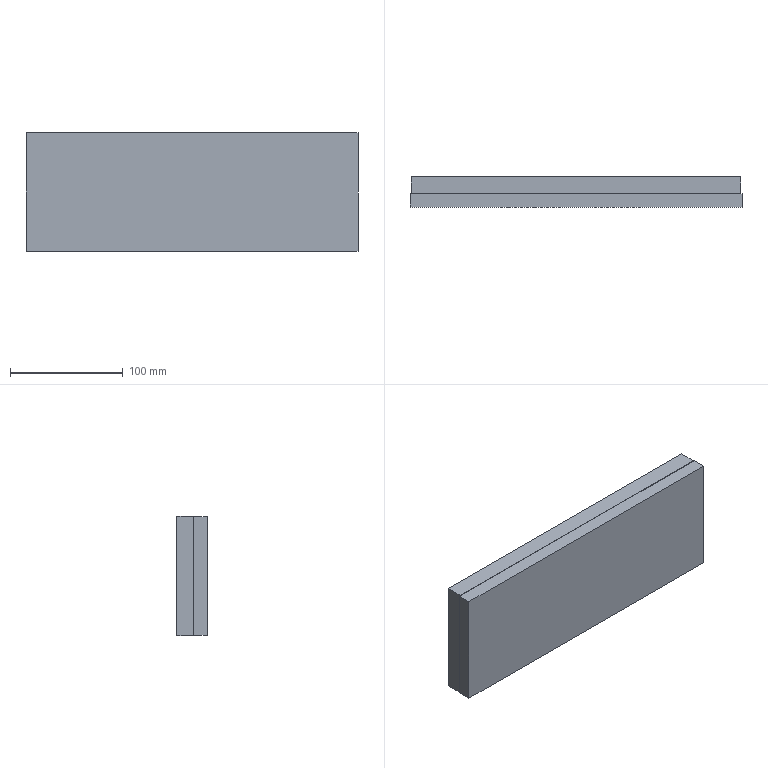CAM job | NX | 3-axis milling, drilling | part box 295 x 27 x 106 mm | stock box 295 x 27 x 106 mm
Tools:
number,name,description,diameter,corner_radius,flute_length,length,flutes
1,D63光面,Milling Tool-5 Parameters,63.0,0.0,50.0,75.0,2
2,D8R0波刀,Milling Tool-5 Parameters,8.0,0.0,50.0,75.0,2
6,D4R0,Milling Tool-5 Parameters,4.0,0.0,50.0,75.0,2
3,D8R0精铣,Milling Tool-5 Parameters,8.0,0.0,50.0,75.0,2
4,DK-D8点孔,Countersink,8.0,0.0,0.0,60.0,2
5,D05钻头,Drilling Tool,5.0,0.0,35.0,50.0,2
8,M6,Drilling Tool,6.0,0.0,35.0,50.0,4
7,DJ-D3倒角,Countersink,3.0,0.0,0.0,60.0,2
4,D10-L40,Milling Tool-5 Parameters,10.0,0.0,30.0,40.0,2
Operations:
program,operation,operation_type,tool,method,geometry_group,spindle_rpm,surface_speed,feed_per_tooth,feed_cut,feed_plunge,cut_length_mm,path_length_mm,cut_time_min,machine_time_min
A1,DRILLING,Operation,DK-D8点孔,METHOD,WORKPIECE_1,2000.0,50.0,0.05,200.0,0.0,30.0,446.986,0.15,0.1917
A1,DRILLING_COPY,Operation,D05钻头,METHOD,WORKPIECE_1,2000.0,50.0,0.05,200.0,0.0,51.0,447.437,0.255,0.2946
A1,DRILLING_COPY_1,Operation,D05钻头,METHOD,WORKPIECE_1,2000.0,50.0,0.05,200.0,0.0,20.0,305.399,0.1,0.1285
A1,DRILLING_COPY_COPY,Operation,M6,METHOD,WORKPIECE_1,300.0,5.0,0.0008,1.0,0.0,45.0,435.437,45.0,45.039
B1,FLOOR_WALL_1,VolumeBased25DMillingOperation,D63光面,METHOD,WORKPIECE_1_1,4000.0,791.0,0.125,1000.0,100.0,4508.198,5634.41,4.508,4.621
B1,FLOOR_WALL_1_COPY,VolumeBased25DMillingOperation,D63光面,METHOD,WORKPIECE_1_1,4000.0,791.0,0.1,800.0,100.0,1122.0,1870.208,1.403,1.477
B1,ADAPTIVE_MILLING_2,CavityMilling,D8R0波刀,METHOD,WORKPIECE_1_1,6500.0,163.0,0.2308,3000.0,100.0,12026.288,12034.288,3.444,3.444
B1,FLOOR_WALL_2,VolumeBased25DMillingOperation,D8R0波刀,METHOD,WORKPIECE_1_1,4500.0,113.0,0.1111,1000.0,100.0,4591.96,4803.179,4.592,4.613
B1,PLANAR_MILL_2,PlanarMilling,DJ-D3倒角,METHOD,WORKPIECE_1_1,3500.0,32.0,0.1429,1000.0,100.0,587.475,989.351,0.5875,0.6277
B1,PLANAR_MILL_3,PlanarMilling,DJ-D3倒角,METHOD,WORKPIECE_1_1,3500.0,32.0,0.1429,1000.0,100.0,461.821,657.821,0.4618,0.4814
B1,FLOOR_WALL_1_COPY_COPY,VolumeBased25DMillingOperation,D63光面,METHOD,WORKPIECE_1_1,4000.0,791.0,0.1,800.0,100.0,1122.0,1870.208,1.403,1.477
G56,FLOOR_WALL_3_COPY,VolumeBased25DMillingOperation,D8R0精铣,METHOD,G56,3500.0,87.0,0.0857,600.0,100.0,1606.938,1899.987,2.678,2.708
G56,FLOOR_WALL_3,VolumeBased25DMillingOperation,D8R0精铣,METHOD,G56,3500.0,87.0,0.0857,600.0,100.0,7170.794,7421.691,11.951,11.976
G57,FLOOR_WALL_4,VolumeBased25DMillingOperation,D8R0精铣,METHOD,G57,4500.0,113.0,0.1111,1000.0,100.0,2652.174,2847.772,2.652,2.672
G57,FLOOR_WALL_4_COPY,VolumeBased25DMillingOperation,D8R0精铣,METHOD,G57,3500.0,87.0,0.1143,800.0,100.0,2654.595,2850.392,3.318,3.338
G57,FLOOR_WALL_5,VolumeBased25DMillingOperation,D8R0精铣,METHOD,G57,3500.0,87.0,0.1143,800.0,100.0,1229.562,1724.911,1.537,1.587
G57,FLOOR_WALL_6,VolumeBased25DMillingOperation,D8R0精铣,METHOD,G57,3500.0,87.0,0.1143,800.0,100.0,2867.751,3374.105,3.585,3.635
G57,PLANAR_MILL_4,PlanarMilling,D8R0精铣,METHOD,G57,3500.0,87.0,0.1143,800.0,100.0,487.323,541.323,0.6092,0.6146
G57,PLANAR_MILL_2_COPY,PlanarMilling,DJ-D3倒角,METHOD,G57,3500.0,32.0,0.1429,1000.0,100.0,587.475,1136.614,0.5875,0.6424
G57,PLANAR_MILL_2_COPY_COPY,PlanarMilling,DJ-D3倒角,METHOD,G57,3500.0,32.0,0.1429,1000.0,100.0,117.155,608.072,0.1172,0.1662
G57,PLANAR_MILL_3_COPY,PlanarMilling,DJ-D3倒角,METHOD,G57,3500.0,32.0,0.1429,1000.0,100.0,555.499,1010.276,0.5555,0.601
G57,PLANAR_MILL_5_COPY,PlanarMilling,DJ-D3倒角,METHOD,G57,3500.0,32.0,0.1429,1000.0,100.0,174.545,365.545,0.1745,0.1936
G57,PLANAR_MILL_5,PlanarMilling,DJ-D3倒角,METHOD,G57,3500.0,32.0,0.1429,1000.0,100.0,262.702,306.702,0.2627,0.2671
F1,FLOOR_WALL_3_COPY_1_COPY,VolumeBased25DMillingOperation,D8R0精铣,METHOD,G58,3500.0,87.0,0.1143,800.0,100.0,3575.353,3610.353,4.469,4.473
F1,FLOOR_WALL_3_COPY_COPY,VolumeBased25DMillingOperation,D8R0精铣,METHOD,G58,3500.0,87.0,0.1429,1000.0,100.0,1602.299,1895.228,1.602,1.632
F1,FLOOR_WALL_3_COPY_COPY_COPY,VolumeBased25DMillingOperation,D8R0精铣,METHOD,G58,4500.0,87.0,0.1143,800.0,100.0,1602.299,1895.348,2.003,2.032
F1,PLANAR_MILL_6,PlanarMilling,D4R0,METHOD,G58,3000.0,37.0,0.0667,400.0,100.0,378.928,691.974,0.9473,0.9786
F1,PLANAR_MILL_6_COPY,PlanarMilling,D4R0,METHOD,G58,3000.0,37.0,0.025,150.0,100.0,41.259,355.512,0.2751,0.3065
F1,PLANAR_MILL_7,PlanarMilling,DJ-D3倒角,METHOD,G58,6000.0,28.0,0.1667,1000.0,100.0,155.988,733.737,0.156,0.2138
F1,PLANAR_MILL_7_COPY,PlanarMilling,DJ-D3倒角,METHOD,G58,6000.0,28.0,0.1667,1000.0,100.0,557.595,814.395,0.5576,0.5833
F1,PLANAR_MILL_7_COPY_COPY,PlanarMilling,DJ-D3倒角,METHOD,G58,6000.0,28.0,0.1667,1000.0,100.0,260.469,297.469,0.2605,0.2642
F1,PLANAR_MILL_7_COPY_COPY_COPY,PlanarMilling,DJ-D3倒角,METHOD,G58,6000.0,28.0,0.1667,1000.0,100.0,390.283,566.283,0.3903,0.4079
G59,FLOOR_WALL_6_COPY,VolumeBased25DMillingOperation,D8R0精铣,METHOD,G59,3500.0,87.0,0.1143,800.0,100.0,1229.856,1274.056,1.537,1.542
G59,PLANAR_MILL_9,PlanarMilling,D8R0精铣,METHOD,G59,3500.0,87.0,0.0857,600.0,100.0,259.771,415.642,0.433,0.4485
G59,FLOOR_WALL_5_COPY,VolumeBased25DMillingOperation,D8R0精铣,METHOD,G59,3500.0,87.0,0.0857,600.0,100.0,1227.675,1723.487,2.046,2.096
G59,PLANAR_MILL_10,PlanarMilling,DJ-D3倒角,METHOD,G59,3500.0,32.0,0.1143,800.0,100.0,221.501,370.841,0.2769,0.2918
G59,PLANAR_MILL_10_COPY,PlanarMilling,DJ-D3倒角,METHOD,G59,3500.0,32.0,0.1143,800.0,100.0,260.702,306.702,0.3259,0.3305
铣孔,PLANAR_MILL_8,PlanarMilling,D4R0,METHOD,铣孔,3500.0,43.0,0.0571,400.0,100.0,471.226,510.226,1.178,1.182
GZ-01,FLOOR_WALL_6_COPY_COPY,VolumeBased25DMillingOperation,D10-L40,METHOD,WORKPIECE,6500.0,87.0,0.1143,4000.0,100.0,69994.164,70718.907,17.498,17.571
GZ-01,FLOOR_WALL_6_COPY_COPY_COPY,VolumeBased25DMillingOperation,D10-L40,METHOD,WORKPIECE,6500.0,87.0,0.1143,1500.0,100.0,4988.257,5022.257,3.325,3.329
GZ-01,FLOOR_WALL_6_COPY_COPY_COPY_COPY,VolumeBased25DMillingOperation,D10-L40,METHOD,WORKPIECE,6500.0,87.0,0.1143,1500.0,100.0,119.728,433.372,0.0798,0.1112
GZ-01,PLANAR_MILL_10_COPY_1,PlanarMilling,DJ-D3倒角,METHOD,WORKPIECE,3500.0,32.0,0.1143,800.0,100.0,64.496,342.874,0.0806,0.1085